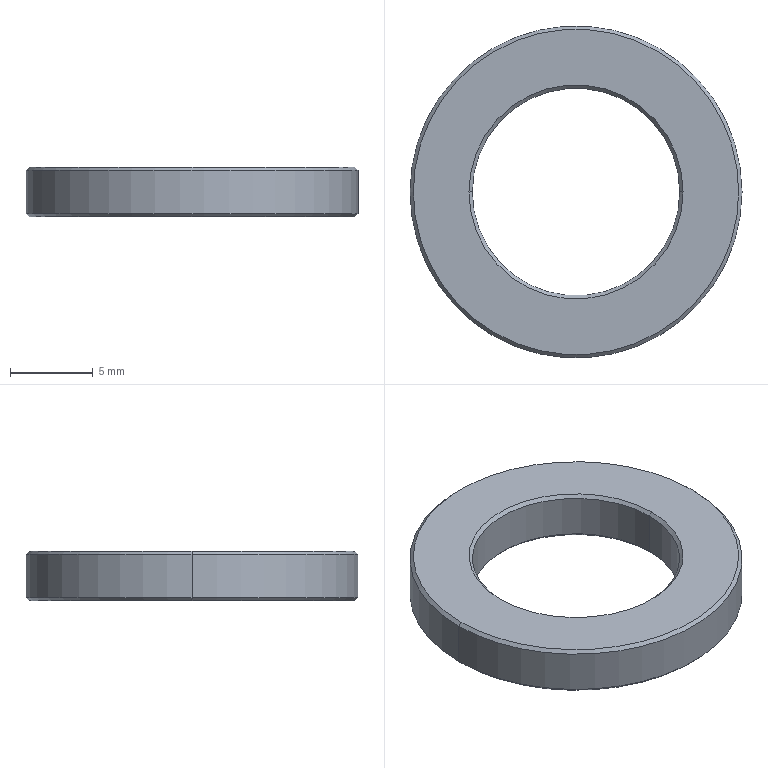Part | SolidWorks | features Chamfer 1, Extrusion 1 | 1 solid | 14 faces | box 20 x 20 x 3 mm | volume 570.238 mm3 | cone 8 | cylinder 4 | plane 2 | commonest cylinder face diameters 12.5 x2 20 x2
STEP:
#1=CARTESIAN_POINT('',(9.8,0.,3.));
#2=VERTEX_POINT('',#1);
#3=CARTESIAN_POINT('',(-9.8,0.,3.));
#4=VERTEX_POINT('',#3);
#5=CARTESIAN_POINT('',(0.,0.,3.));
#6=DIRECTION('',(0.,0.,1.));
#7=DIRECTION('',(1.,0.,0.));
#8=AXIS2_PLACEMENT_3D('',#5,#6,#7);
#9=CIRCLE('',#8,9.8);
#10=EDGE_CURVE('',#2,#4,#9,.T.);
#11=ORIENTED_EDGE('',*,*,#10,.F.);
#12=CARTESIAN_POINT('',(10.,0.,2.8));
#13=VERTEX_POINT('',#12);
#14=CARTESIAN_POINT('',(9.8,0.,3.));
#15=DIRECTION('',(0.7071,0.,-0.7071));
#16=VECTOR('',#15,1000.);
#17=LINE('',#14,#16);
#18=EDGE_CURVE('',#2,#13,#17,.T.);
#19=ORIENTED_EDGE('',*,*,#18,.T.);
#20=CARTESIAN_POINT('',(-10.,0.,2.8));
#21=VERTEX_POINT('',#20);
#22=CARTESIAN_POINT('',(0.,0.,2.8));
#23=DIRECTION('',(0.,0.,-1.));
#24=DIRECTION('',(1.,0.,0.));
#25=AXIS2_PLACEMENT_3D('',#22,#23,#24);
#26=CIRCLE('',#25,10.);
#27=EDGE_CURVE('',#21,#13,#26,.T.);
#28=ORIENTED_EDGE('',*,*,#27,.F.);
#29=CARTESIAN_POINT('',(-9.8,0.,3.));
#30=DIRECTION('',(-0.7071,0.,-0.7071));
#31=VECTOR('',#30,1000.);
#32=LINE('',#29,#31);
#33=EDGE_CURVE('',#4,#21,#32,.T.);
#34=ORIENTED_EDGE('',*,*,#33,.F.);
#35=EDGE_LOOP('',(#11,#19,#28,#34));
#36=FACE_OUTER_BOUND('',#35,.T.);
#37=CARTESIAN_POINT('',(0.,0.,3.));
#38=DIRECTION('',(0.,0.,-1.));
#39=DIRECTION('',(-1.,0.,0.));
#40=AXIS2_PLACEMENT_3D('',#37,#38,#39);
#41=CONICAL_SURFACE('',#40,9.8,0.7854);
#42=ADVANCED_FACE('',(#36),#41,.T.);
#43=CARTESIAN_POINT('',(-6.25,0.,2.8));
#44=VERTEX_POINT('',#43);
#45=CARTESIAN_POINT('',(6.25,0.,2.8));
#46=VERTEX_POINT('',#45);
#47=CARTESIAN_POINT('',(0.,0.,2.8));
#48=DIRECTION('',(0.,0.,1.));
#49=DIRECTION('',(1.,0.,0.));
#50=AXIS2_PLACEMENT_3D('',#47,#48,#49);
#51=CIRCLE('',#50,6.25);
#52=EDGE_CURVE('',#44,#46,#51,.T.);
#53=ORIENTED_EDGE('',*,*,#52,.F.);
#54=CARTESIAN_POINT('',(-6.45,0.,3.));
#55=VERTEX_POINT('',#54);
#56=CARTESIAN_POINT('',(-6.25,0.,2.8));
#57=DIRECTION('',(-0.7071,0.,0.7071));
#58=VECTOR('',#57,1000.);
#59=LINE('',#56,#58);
#60=EDGE_CURVE('',#44,#55,#59,.T.);
#61=ORIENTED_EDGE('',*,*,#60,.T.);
#62=CARTESIAN_POINT('',(6.45,0.,3.));
#63=VERTEX_POINT('',#62);
#64=CARTESIAN_POINT('',(0.,0.,3.));
#65=DIRECTION('',(0.,0.,-1.));
#66=DIRECTION('',(1.,0.,0.));
#67=AXIS2_PLACEMENT_3D('',#64,#65,#66);
#68=CIRCLE('',#67,6.45);
#69=EDGE_CURVE('',#63,#55,#68,.T.);
#70=ORIENTED_EDGE('',*,*,#69,.F.);
#71=CARTESIAN_POINT('',(6.25,0.,2.8));
#72=DIRECTION('',(0.7071,0.,0.7071));
#73=VECTOR('',#72,1000.);
#74=LINE('',#71,#73);
#75=EDGE_CURVE('',#46,#63,#74,.T.);
#76=ORIENTED_EDGE('',*,*,#75,.F.);
#77=EDGE_LOOP('',(#53,#61,#70,#76));
#78=FACE_OUTER_BOUND('',#77,.T.);
#79=CARTESIAN_POINT('',(0.,0.,2.8));
#80=DIRECTION('',(0.,0.,1.));
#81=DIRECTION('',(1.,0.,0.));
#82=AXIS2_PLACEMENT_3D('',#79,#80,#81);
#83=CONICAL_SURFACE('',#82,6.25,0.7854);
#84=ADVANCED_FACE('',(#78),#83,.F.);
#85=CARTESIAN_POINT('',(-9.8,0.,0.));
#86=VERTEX_POINT('',#85);
#87=CARTESIAN_POINT('',(9.8,0.,0.));
#88=VERTEX_POINT('',#87);
#89=CARTESIAN_POINT('',(0.,0.,0.));
#90=DIRECTION('',(0.,0.,-1.));
#91=DIRECTION('',(1.,0.,0.));
#92=AXIS2_PLACEMENT_3D('',#89,#90,#91);
#93=CIRCLE('',#92,9.8);
#94=EDGE_CURVE('',#86,#88,#93,.T.);
#95=ORIENTED_EDGE('',*,*,#94,.F.);
#96=CARTESIAN_POINT('',(-10.,0.,0.2));
#97=VERTEX_POINT('',#96);
#98=CARTESIAN_POINT('',(-10.,0.,0.2));
#99=DIRECTION('',(-0.7071,0.,0.7071));
#100=VECTOR('',#99,1000.);
#101=LINE('',#98,#100);
#102=EDGE_CURVE('',#86,#97,#101,.T.);
#103=ORIENTED_EDGE('',*,*,#102,.T.);
#104=CARTESIAN_POINT('',(10.,0.,0.2));
#105=VERTEX_POINT('',#104);
#106=CARTESIAN_POINT('',(0.,0.,0.2));
#107=DIRECTION('',(0.,0.,1.));
#108=DIRECTION('',(1.,0.,0.));
#109=AXIS2_PLACEMENT_3D('',#106,#107,#108);
#110=CIRCLE('',#109,10.);
#111=EDGE_CURVE('',#105,#97,#110,.T.);
#112=ORIENTED_EDGE('',*,*,#111,.F.);
#113=CARTESIAN_POINT('',(10.,0.,0.2));
#114=DIRECTION('',(0.7071,0.,0.7071));
#115=VECTOR('',#114,1000.);
#116=LINE('',#113,#115);
#117=EDGE_CURVE('',#88,#105,#116,.T.);
#118=ORIENTED_EDGE('',*,*,#117,.F.);
#119=EDGE_LOOP('',(#95,#103,#112,#118));
#120=FACE_OUTER_BOUND('',#119,.T.);
#121=CARTESIAN_POINT('',(0.,0.,0.2));
#122=DIRECTION('',(0.,0.,1.));
#123=DIRECTION('',(1.,0.,0.));
#124=AXIS2_PLACEMENT_3D('',#121,#122,#123);
#125=CONICAL_SURFACE('',#124,10.,0.7854);
#126=ADVANCED_FACE('',(#120),#125,.T.);
#127=CARTESIAN_POINT('',(6.25,0.,0.2));
#128=VERTEX_POINT('',#127);
#129=CARTESIAN_POINT('',(-6.25,0.,0.2));
#130=VERTEX_POINT('',#129);
#131=CARTESIAN_POINT('',(0.,0.,0.2));
#132=DIRECTION('',(0.,0.,-1.));
#133=DIRECTION('',(1.,0.,0.));
#134=AXIS2_PLACEMENT_3D('',#131,#132,#133);
#135=CIRCLE('',#134,6.25);
#136=EDGE_CURVE('',#128,#130,#135,.T.);
#137=ORIENTED_EDGE('',*,*,#136,.F.);
#138=CARTESIAN_POINT('',(6.45,0.,0.));
#139=VERTEX_POINT('',#138);
#140=CARTESIAN_POINT('',(6.45,0.,0.));
#141=DIRECTION('',(0.7071,0.,-0.7071));
#142=VECTOR('',#141,1000.);
#143=LINE('',#140,#142);
#144=EDGE_CURVE('',#128,#139,#143,.T.);
#145=ORIENTED_EDGE('',*,*,#144,.T.);
#146=CARTESIAN_POINT('',(-6.45,0.,0.));
#147=VERTEX_POINT('',#146);
#148=CARTESIAN_POINT('',(0.,0.,0.));
#149=DIRECTION('',(0.,0.,1.));
#150=DIRECTION('',(1.,0.,0.));
#151=AXIS2_PLACEMENT_3D('',#148,#149,#150);
#152=CIRCLE('',#151,6.45);
#153=EDGE_CURVE('',#147,#139,#152,.T.);
#154=ORIENTED_EDGE('',*,*,#153,.F.);
#155=CARTESIAN_POINT('',(-6.45,0.,0.));
#156=DIRECTION('',(-0.7071,0.,-0.7071));
#157=VECTOR('',#156,1000.);
#158=LINE('',#155,#157);
#159=EDGE_CURVE('',#130,#147,#158,.T.);
#160=ORIENTED_EDGE('',*,*,#159,.F.);
#161=EDGE_LOOP('',(#137,#145,#154,#160));
#162=FACE_OUTER_BOUND('',#161,.T.);
#163=CARTESIAN_POINT('',(0.,0.,0.));
#164=DIRECTION('',(0.,0.,-1.));
#165=DIRECTION('',(-1.,0.,0.));
#166=AXIS2_PLACEMENT_3D('',#163,#164,#165);
#167=CONICAL_SURFACE('',#166,6.45,0.7854);
#168=ADVANCED_FACE('',(#162),#167,.F.);
#169=ORIENTED_EDGE('',*,*,#52,.T.);
#170=CARTESIAN_POINT('',(6.25,0.,3.));
#171=DIRECTION('',(0.,0.,-1.));
#172=VECTOR('',#171,1000.);
#173=LINE('',#170,#172);
#174=EDGE_CURVE('',#46,#128,#173,.T.);
#175=ORIENTED_EDGE('',*,*,#174,.T.);
#176=ORIENTED_EDGE('',*,*,#136,.T.);
#177=CARTESIAN_POINT('',(-6.25,0.,3.));
#178=DIRECTION('',(0.,0.,-1.));
#179=VECTOR('',#178,1000.);
#180=LINE('',#177,#179);
#181=EDGE_CURVE('',#44,#130,#180,.T.);
#182=ORIENTED_EDGE('',*,*,#181,.F.);
#183=EDGE_LOOP('',(#169,#175,#176,#182));
#184=FACE_OUTER_BOUND('',#183,.T.);
#185=CARTESIAN_POINT('',(0.,0.,3.));
#186=DIRECTION('',(0.,0.,-1.));
#187=DIRECTION('',(-1.,0.,0.));
#188=AXIS2_PLACEMENT_3D('',#185,#186,#187);
#189=CYLINDRICAL_SURFACE('',#188,6.25);
#190=ADVANCED_FACE('',(#184),#189,.F.);
#191=ORIENTED_EDGE('',*,*,#27,.T.);
#192=CARTESIAN_POINT('',(10.,0.,3.));
#193=DIRECTION('',(0.,0.,-1.));
#194=VECTOR('',#193,1000.);
#195=LINE('',#192,#194);
#196=EDGE_CURVE('',#13,#105,#195,.T.);
#197=ORIENTED_EDGE('',*,*,#196,.T.);
#198=ORIENTED_EDGE('',*,*,#111,.T.);
#199=CARTESIAN_POINT('',(-10.,0.,3.));
#200=DIRECTION('',(0.,0.,-1.));
#201=VECTOR('',#200,1000.);
#202=LINE('',#199,#201);
#203=EDGE_CURVE('',#21,#97,#202,.T.);
#204=ORIENTED_EDGE('',*,*,#203,.F.);
#205=EDGE_LOOP('',(#191,#197,#198,#204));
#206=FACE_OUTER_BOUND('',#205,.T.);
#207=CARTESIAN_POINT('',(0.,0.,3.));
#208=DIRECTION('',(0.,0.,-1.));
#209=DIRECTION('',(-1.,0.,0.));
#210=AXIS2_PLACEMENT_3D('',#207,#208,#209);
#211=CYLINDRICAL_SURFACE('',#210,10.);
#212=ADVANCED_FACE('',(#206),#211,.T.);
#213=ORIENTED_EDGE('',*,*,#69,.T.);
#214=CARTESIAN_POINT('',(0.,0.,3.));
#215=DIRECTION('',(0.,0.,-1.));
#216=DIRECTION('',(1.,0.,0.));
#217=AXIS2_PLACEMENT_3D('',#214,#215,#216);
#218=CIRCLE('',#217,6.45);
#219=EDGE_CURVE('',#55,#63,#218,.T.);
#220=ORIENTED_EDGE('',*,*,#219,.T.);
#221=EDGE_LOOP('',(#213,#220));
#222=FACE_BOUND('',#221,.T.);
#223=CARTESIAN_POINT('',(0.,0.,3.));
#224=DIRECTION('',(0.,0.,1.));
#225=DIRECTION('',(1.,0.,0.));
#226=AXIS2_PLACEMENT_3D('',#223,#224,#225);
#227=CIRCLE('',#226,9.8);
#228=EDGE_CURVE('',#4,#2,#227,.T.);
#229=ORIENTED_EDGE('',*,*,#228,.T.);
#230=ORIENTED_EDGE('',*,*,#10,.T.);
#231=EDGE_LOOP('',(#229,#230));
#232=FACE_OUTER_BOUND('',#231,.T.);
#233=CARTESIAN_POINT('',(0.,0.,3.));
#234=DIRECTION('',(0.,0.,1.));
#235=DIRECTION('',(1.,0.,0.));
#236=AXIS2_PLACEMENT_3D('',#233,#234,#235);
#237=PLANE('',#236);
#238=ADVANCED_FACE('',(#222,#232),#237,.T.);
#239=ORIENTED_EDGE('',*,*,#153,.T.);
#240=CARTESIAN_POINT('',(0.,0.,0.));
#241=DIRECTION('',(0.,0.,1.));
#242=DIRECTION('',(1.,0.,0.));
#243=AXIS2_PLACEMENT_3D('',#240,#241,#242);
#244=CIRCLE('',#243,6.45);
#245=EDGE_CURVE('',#139,#147,#244,.T.);
#246=ORIENTED_EDGE('',*,*,#245,.T.);
#247=EDGE_LOOP('',(#239,#246));
#248=FACE_BOUND('',#247,.T.);
#249=CARTESIAN_POINT('',(0.,0.,0.));
#250=DIRECTION('',(0.,0.,-1.));
#251=DIRECTION('',(1.,0.,0.));
#252=AXIS2_PLACEMENT_3D('',#249,#250,#251);
#253=CIRCLE('',#252,9.8);
#254=EDGE_CURVE('',#88,#86,#253,.T.);
#255=ORIENTED_EDGE('',*,*,#254,.T.);
#256=ORIENTED_EDGE('',*,*,#94,.T.);
#257=EDGE_LOOP('',(#255,#256));
#258=FACE_OUTER_BOUND('',#257,.T.);
#259=CARTESIAN_POINT('',(0.,0.,0.));
#260=DIRECTION('',(0.,0.,1.));
#261=DIRECTION('',(1.,0.,0.));
#262=AXIS2_PLACEMENT_3D('',#259,#260,#261);
#263=PLANE('',#262);
#264=ADVANCED_FACE('',(#248,#258),#263,.F.);
#265=ORIENTED_EDGE('',*,*,#196,.F.);
#266=CARTESIAN_POINT('',(0.,0.,2.8));
#267=DIRECTION('',(0.,0.,-1.));
#268=DIRECTION('',(1.,0.,0.));
#269=AXIS2_PLACEMENT_3D('',#266,#267,#268);
#270=CIRCLE('',#269,10.);
#271=EDGE_CURVE('',#13,#21,#270,.T.);
#272=ORIENTED_EDGE('',*,*,#271,.T.);
#273=ORIENTED_EDGE('',*,*,#203,.T.);
#274=CARTESIAN_POINT('',(0.,0.,0.2));
#275=DIRECTION('',(0.,0.,1.));
#276=DIRECTION('',(1.,0.,0.));
#277=AXIS2_PLACEMENT_3D('',#274,#275,#276);
#278=CIRCLE('',#277,10.);
#279=EDGE_CURVE('',#97,#105,#278,.T.);
#280=ORIENTED_EDGE('',*,*,#279,.T.);
#281=EDGE_LOOP('',(#265,#272,#273,#280));
#282=FACE_OUTER_BOUND('',#281,.T.);
#283=CARTESIAN_POINT('',(0.,0.,3.));
#284=DIRECTION('',(0.,0.,-1.));
#285=DIRECTION('',(-1.,0.,0.));
#286=AXIS2_PLACEMENT_3D('',#283,#284,#285);
#287=CYLINDRICAL_SURFACE('',#286,10.);
#288=ADVANCED_FACE('',(#282),#287,.T.);
#289=ORIENTED_EDGE('',*,*,#174,.F.);
#290=CARTESIAN_POINT('',(0.,0.,2.8));
#291=DIRECTION('',(0.,0.,1.));
#292=DIRECTION('',(1.,0.,0.));
#293=AXIS2_PLACEMENT_3D('',#290,#291,#292);
#294=CIRCLE('',#293,6.25);
#295=EDGE_CURVE('',#46,#44,#294,.T.);
#296=ORIENTED_EDGE('',*,*,#295,.T.);
#297=ORIENTED_EDGE('',*,*,#181,.T.);
#298=CARTESIAN_POINT('',(0.,0.,0.2));
#299=DIRECTION('',(0.,0.,-1.));
#300=DIRECTION('',(1.,0.,0.));
#301=AXIS2_PLACEMENT_3D('',#298,#299,#300);
#302=CIRCLE('',#301,6.25);
#303=EDGE_CURVE('',#130,#128,#302,.T.);
#304=ORIENTED_EDGE('',*,*,#303,.T.);
#305=EDGE_LOOP('',(#289,#296,#297,#304));
#306=FACE_OUTER_BOUND('',#305,.T.);
#307=CARTESIAN_POINT('',(0.,0.,3.));
#308=DIRECTION('',(0.,0.,-1.));
#309=DIRECTION('',(-1.,0.,0.));
#310=AXIS2_PLACEMENT_3D('',#307,#308,#309);
#311=CYLINDRICAL_SURFACE('',#310,6.25);
#312=ADVANCED_FACE('',(#306),#311,.F.);
#313=ORIENTED_EDGE('',*,*,#144,.F.);
#314=ORIENTED_EDGE('',*,*,#303,.F.);
#315=ORIENTED_EDGE('',*,*,#159,.T.);
#316=ORIENTED_EDGE('',*,*,#245,.F.);
#317=EDGE_LOOP('',(#313,#314,#315,#316));
#318=FACE_OUTER_BOUND('',#317,.T.);
#319=CARTESIAN_POINT('',(0.,0.,0.));
#320=DIRECTION('',(0.,0.,-1.));
#321=DIRECTION('',(-1.,0.,0.));
#322=AXIS2_PLACEMENT_3D('',#319,#320,#321);
#323=CONICAL_SURFACE('',#322,6.45,0.7854);
#324=ADVANCED_FACE('',(#318),#323,.F.);
#325=ORIENTED_EDGE('',*,*,#102,.F.);
#326=ORIENTED_EDGE('',*,*,#254,.F.);
#327=ORIENTED_EDGE('',*,*,#117,.T.);
#328=ORIENTED_EDGE('',*,*,#279,.F.);
#329=EDGE_LOOP('',(#325,#326,#327,#328));
#330=FACE_OUTER_BOUND('',#329,.T.);
#331=CARTESIAN_POINT('',(0.,0.,0.2));
#332=DIRECTION('',(0.,0.,1.));
#333=DIRECTION('',(1.,0.,0.));
#334=AXIS2_PLACEMENT_3D('',#331,#332,#333);
#335=CONICAL_SURFACE('',#334,10.,0.7854);
#336=ADVANCED_FACE('',(#330),#335,.T.);
#337=ORIENTED_EDGE('',*,*,#60,.F.);
#338=ORIENTED_EDGE('',*,*,#295,.F.);
#339=ORIENTED_EDGE('',*,*,#75,.T.);
#340=ORIENTED_EDGE('',*,*,#219,.F.);
#341=EDGE_LOOP('',(#337,#338,#339,#340));
#342=FACE_OUTER_BOUND('',#341,.T.);
#343=CARTESIAN_POINT('',(0.,0.,2.8));
#344=DIRECTION('',(0.,0.,1.));
#345=DIRECTION('',(1.,0.,0.));
#346=AXIS2_PLACEMENT_3D('',#343,#344,#345);
#347=CONICAL_SURFACE('',#346,6.25,0.7854);
#348=ADVANCED_FACE('',(#342),#347,.F.);
#349=ORIENTED_EDGE('',*,*,#18,.F.);
#350=ORIENTED_EDGE('',*,*,#228,.F.);
#351=ORIENTED_EDGE('',*,*,#33,.T.);
#352=ORIENTED_EDGE('',*,*,#271,.F.);
#353=EDGE_LOOP('',(#349,#350,#351,#352));
#354=FACE_OUTER_BOUND('',#353,.T.);
#355=CARTESIAN_POINT('',(0.,0.,3.));
#356=DIRECTION('',(0.,0.,-1.));
#357=DIRECTION('',(-1.,0.,0.));
#358=AXIS2_PLACEMENT_3D('',#355,#356,#357);
#359=CONICAL_SURFACE('',#358,9.8,0.7854);
#360=ADVANCED_FACE('',(#354),#359,.T.);
#361=CLOSED_SHELL('',(#42,#84,#126,#168,#190,#212,#238,#264,#288,#312,#324,#336,#348,#360));
#362=MANIFOLD_SOLID_BREP('',#361);
#363=CARTESIAN_POINT('',(0.,0.,0.));
#364=DIRECTION('',(0.,0.,1.));
#365=DIRECTION('',(1.,0.,0.));
#366=AXIS2_PLACEMENT_3D('',#363,#364,#365);
#367=(LENGTH_UNIT()NAMED_UNIT(*)SI_UNIT(.MILLI.,.METRE.));
#368=UNCERTAINTY_MEASURE_WITH_UNIT(LENGTH_MEASURE(0.00001),#367,'','');
#369=(NAMED_UNIT(*)PLANE_ANGLE_UNIT()SI_UNIT($,.RADIAN.));
#370=(NAMED_UNIT(*)SI_UNIT($,.STERADIAN.)SOLID_ANGLE_UNIT());
#371=(GEOMETRIC_REPRESENTATION_CONTEXT(3)GLOBAL_UNCERTAINTY_ASSIGNED_CONTEXT((#368))GLOBAL_UNIT_ASSIGNED_CONTEXT((#367,#369,#370))REPRESENTATION_CONTEXT('',''));
#372=ADVANCED_BREP_SHAPE_REPRESENTATION('',(#362,#366),#371);